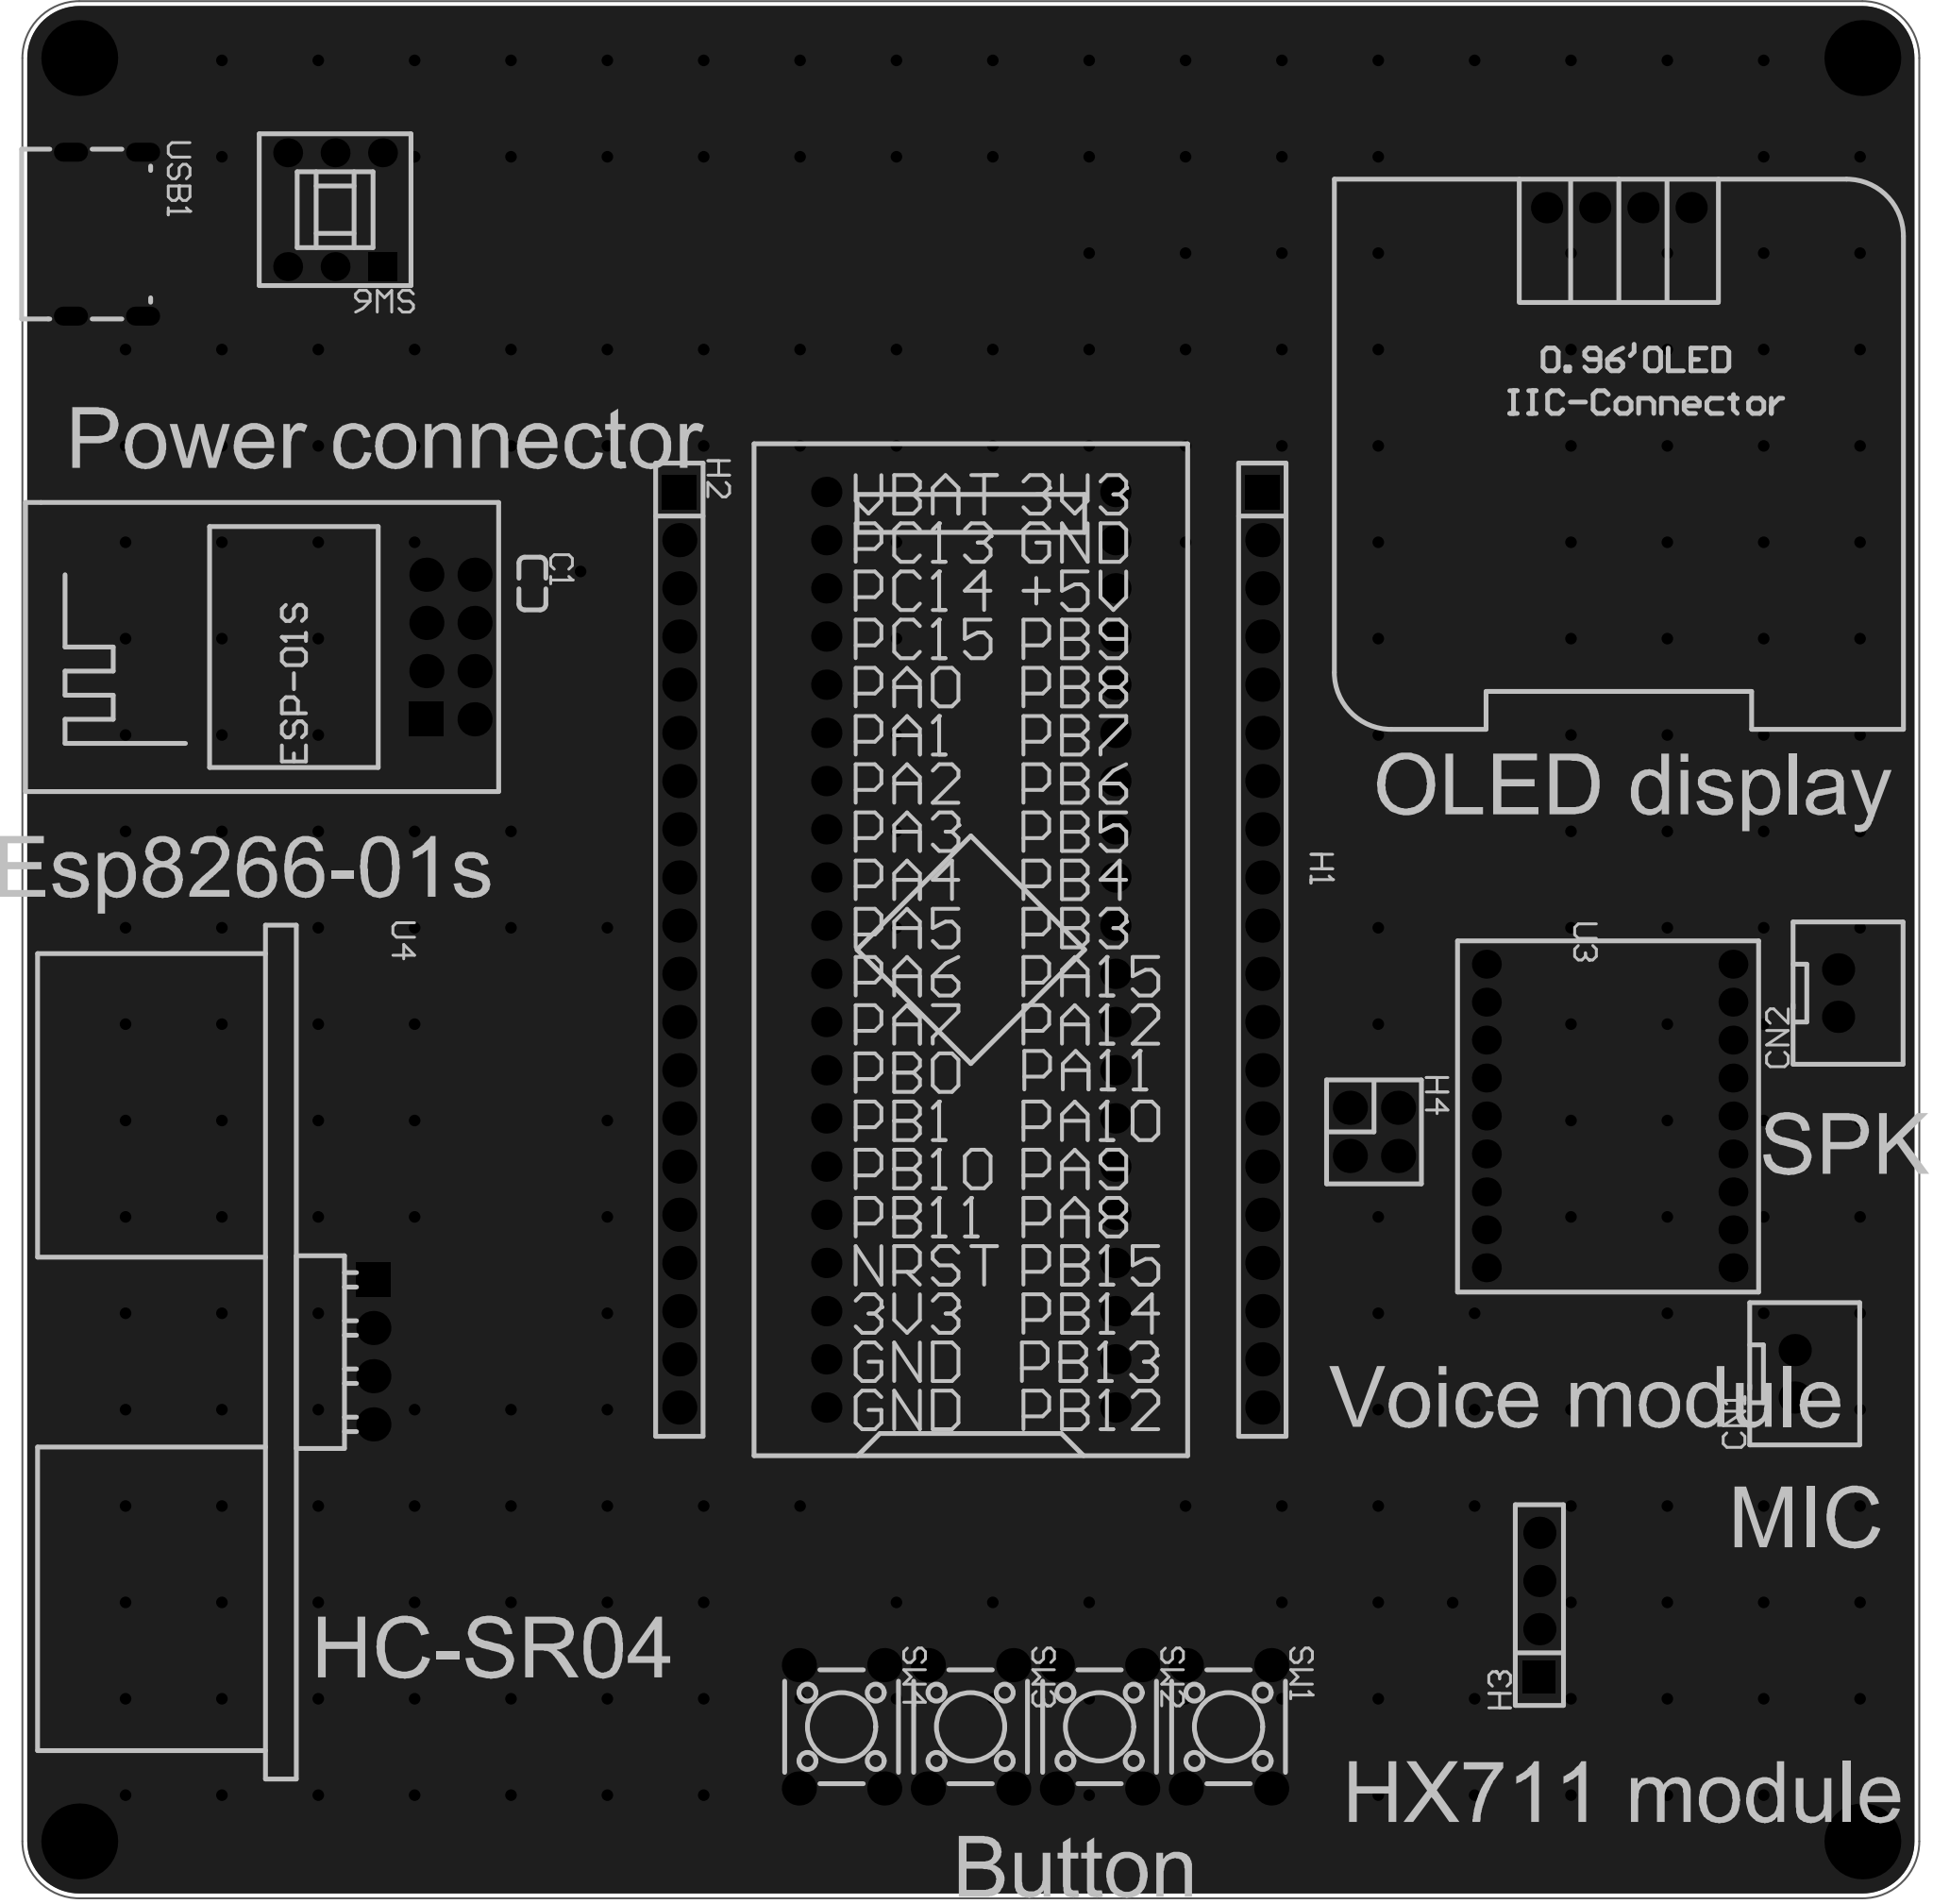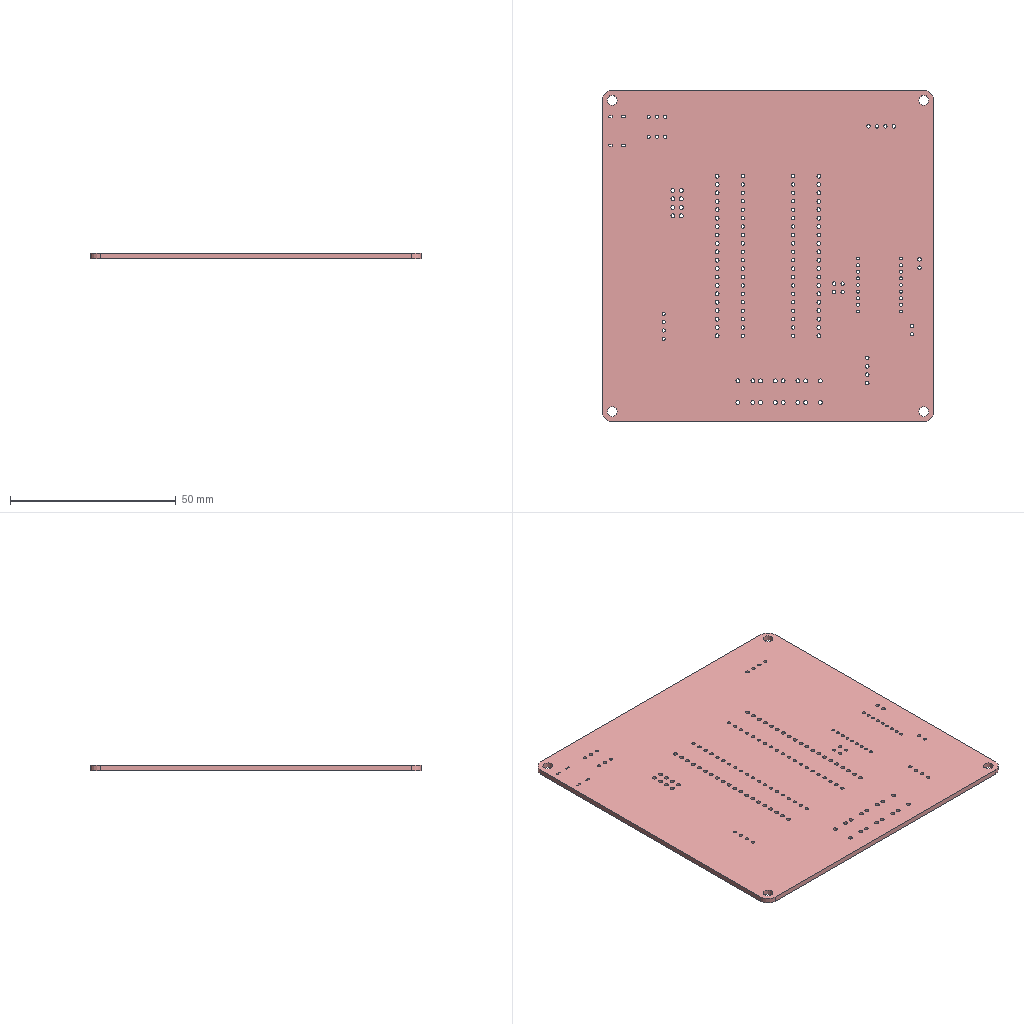Circuit board layout | Altium Designer | box 100 x 100 x 1.6 mm
Layer stack:
# Altium Designer layer stack of  (unit mm; dielectric type: 0 none, 1 core, 2 prepreg, 3 surface material)
index,name,kind,layer,copper_thickness_mm,dielectric_type,dielectric_thickness_mm,dielectric_material,dielectric_constant
0,Top Paste Mask Layer,other,,,,,,
1,Top Silkscreen Layer,other,,,,,,
2,Top Solder Mask Layer,dielectric,,,3,0.01,,3.3
3,Top Layer,copper,Top Layer,0.035,,,,
4,Dielectric1,dielectric,,,3,1.51,FR4,4.5
5,Bottom Layer,copper,Bottom Layer,0.035,,,,
6,Bottom Solder Mask Layer,dielectric,,,3,0.01,,3.3
7,Bottom Silkscreen Layer,other,,,,,,
8,Bottom Paste Mask Layer,other,,,,,,
# drill layer pairs: low layer,high layer
drill_pair,Top Layer,Bottom Layer
Part placement:
Designator,Comment,Layer,Footprint,Center-X(mm),Center-Y(mm),Rotation
U1,STM32F103C8T6-Card,TopLayer,CONN-TH_L53.3-W22.9_STM32F103C8T6-CARD,141.351,130.937,90
U2,ESP-01S,TopLayer,WIFIM-TH_ESP-01S,113.919,146.893,90
OLED1,,TopLayer,0.96OLED_4P,175.514,170.053,0
SW1,,TopLayer,SW-TH_4P-L6.0-W6.0-P4.50-LS6.5,154.936,89.979,270
SW2,,TopLayer,SW-TH_4P-L6.0-W6.0-P4.50-LS6.5,148.136,89.979,270
SW3,,TopLayer,SW-TH_4P-L6.0-W6.0-P4.50-LS6.5,141.337,89.979,270
SW4,,TopLayer,SW-TH_4P-L6.0-W6.0-P4.50-LS6.5,134.537,89.979,270
CN1,XH2.54*2P_Through-hole,TopLayer,CONN-TH_2P-P2.50-XH2.54-2P,184.785,108.585,90
CN2,XH2.54*2P_Through-hole,TopLayer,CONN-TH_2P-P2.50-XH2.54-2P,187.071,128.651,90
U3,CON2.0MM-PAD-18,TopLayer,CONN-TH_18P-P2.00_C9900078766,175.029,122.174,270
C1,100nF,TopLayer,C0603,118.237,150.241,270
H2,,TopLayer,HDR-TH_20P-P2.54-V-F,125.984,130.937,270
H3,,TopLayer,HDR-TH_4P-P2.54-V-F,171.323,96.393,90
H4,,TopLayer,HDR-TH_4P-P2.54-V-F-R2-C2-S2.54,162.604,121.335,270
H1,,TopLayer,HDR-TH_20P-P2.54-V-F,156.718,130.937,270
SW6,PS081-06L135D1-JF-G,TopLayer,SW-TH_6P-L8.0-W8.0-P2.50-TL,107.836,169.945,180
U4,HC-SR04,TopLayer,TH_HC-SR04V,109.855,109.728,270
USB1,TYPEC-250D-BCP6,TopLayer,USB-C-SMD_TYPEC-250D-BCP6,96.012,168.656,270
Pad and via stacks:
# Altium Designer via and pad stacks of  (unit mm). Each distinct definition once, with the count of objects using it.
# via: kind,start_layer,end_layer,hole_mm,diameter_mm,mode(0 simple;1 top-mid-bottom;2 full stack),diameter_per_layer,count,example_net
# pad: kind,layer,hole_mm,hole_type(0 round;1 square;2 slot),plating,top_size,top_shape(1 round;2 rect;3 octagon;9 rounded rect),mid_size,bottom_size,mode,footprint,size_per_layer,count,example
pad,Multi-Layer,3,0,plated,4x4,1,4x4,4x4,0,,,4,1
pad,Multi-Layer,1,0,plated,1.6x1.6,1,1.6x1.6,1.6x1.6,0,CONN-TH_L53.3-W22.9_STM32F103C8T6-CARD,,40,U1.1
pad,Multi-Layer,1.2,0,plated,1.8x1.8,2,1.8x1.8,1.8x1.8,0,WIFIM-TH_ESP-01S,,1,U2.1
pad,Multi-Layer,1.2,0,plated,1.8x1.8,1,1.8x1.8,1.8x1.8,0,WIFIM-TH_ESP-01S,,7,U2.2
pad,Multi-Layer,1,0,plated,1.65x1.65,1,1.65x1.65,1.65x1.65,0,0.96OLED_4P,,4,OLED1.4
pad,Multi-Layer,1.2,0,plated,1.8x1.8,1,1.8x1.8,1.8x1.8,0,SW-TH_4P-L6.0-W6.0-P4.50-LS6.5,,16,SW1.1
pad,Multi-Layer,1.05,0,plated,1.7x1.7,1,1.7x1.7,1.7x1.7,0,CONN-TH_2P-P2.50-XH2.54-2P,,4,CN1.2
pad,Multi-Layer,0.9,0,plated,1.524x1.524,1,1.524x1.524,1.524x1.524,0,CONN-TH_18P-P2.00_C9900078766,,18,U3.1
pad,Multi-Layer,1.2,0,plated,1.8x1.8,2,1.8x1.8,1.8x1.8,0,HDR-TH_20P-P2.54-V-F,,2,H2.1
pad,Multi-Layer,1.2,0,plated,1.8x1.8,1,1.8x1.8,1.8x1.8,0,HDR-TH_20P-P2.54-V-F,,38,H2.2
pad,Multi-Layer,1.1,0,plated,1.7x1.7,2,1.7x1.7,1.7x1.7,0,HDR-TH_4P-P2.54-V-F,,1,H3.1
pad,Multi-Layer,1.1,0,plated,1.7x1.7,1,1.7x1.7,1.7x1.7,0,HDR-TH_4P-P2.54-V-F,,3,H3.2
pad,Multi-Layer,1,0,plated,1.8x1.8,1,1.8x1.8,1.8x1.8,0,HDR-TH_4P-P2.54-V-F-R2-C2-S2.54,,4,H4.4
pad,Multi-Layer,1,0,plated,1.524x1.524,1,1.524x1.524,1.524x1.524,0,SW-TH_6P-L8.0-W8.0-P2.50-TL,,5,SW6.4
pad,Multi-Layer,1,0,plated,1.524x1.524,2,1.524x1.524,1.524x1.524,0,SW-TH_6P-L8.0-W8.0-P2.50-TL,,1,SW6.1
pad,Multi-Layer,1.001,0,plated,1.8x1.8,1,1.8x1.8,1.8x1.8,0,TH_HC-SR04V,,3,U4.4
pad,Multi-Layer,1.001,0,plated,1.8x1.8,2,1.8x1.8,1.8x1.8,0,TH_HC-SR04V,,1,U4.1
pad,Multi-Layer,0.5,2,plated,1x1.8,1,1x1.8,1x1.8,0,USB-C-SMD_TYPEC-250D-BCP6,,4,USB1.1
pad,Top Layer,0,0,plated,0.8x0.9,2,0.8x0.9,0.8x0.9,0,C0603,,2,C1.2
pad,Top Layer,0,0,plated,0.75x1.6,2,0.75x1.6,0.75x1.6,0,USB-C-SMD_TYPEC-250D-BCP6,,6,USB1.B12
via,Top Layer,Bottom Layer,0.3048,0.61,0,,238,PB5_SCK
Copper pours:
name,layer,net,type(0 solid;1 hatched;2 none)
Bottom Layer-GND,Bottom Layer,GND,0
Top Layer-GND,Top Layer,GND,0